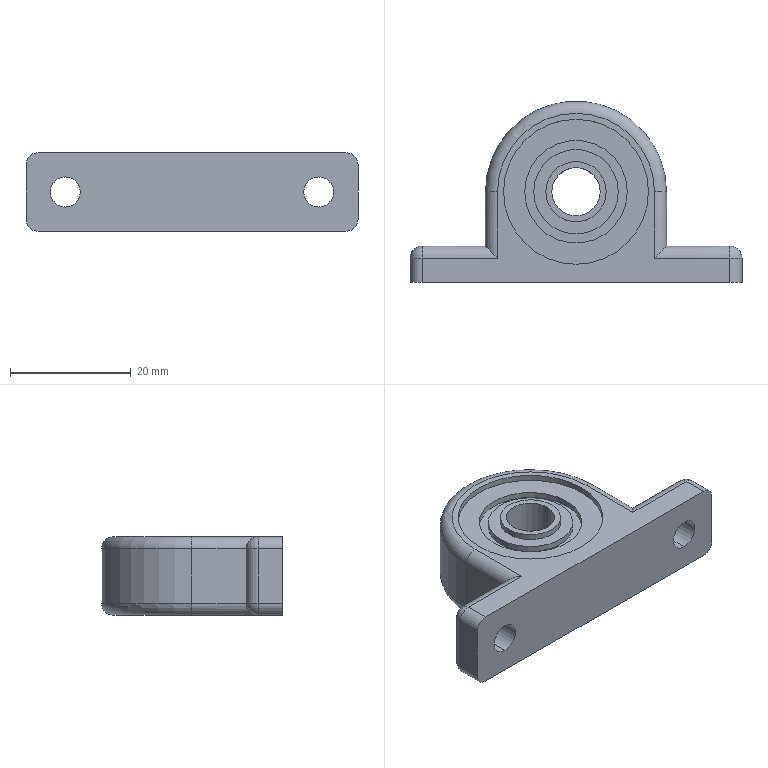Part | STEP file | U-type bearing support 8 | 1 solid | 60 faces | box 55 x 30 x 13 mm | volume 10419 mm3 | cylinder 37 | plane 17 | sphere 4 | torus 2 | commonest cylinder face diameters 4 x14 5 x4 10 x4 14 x4 17 x4 24 x4